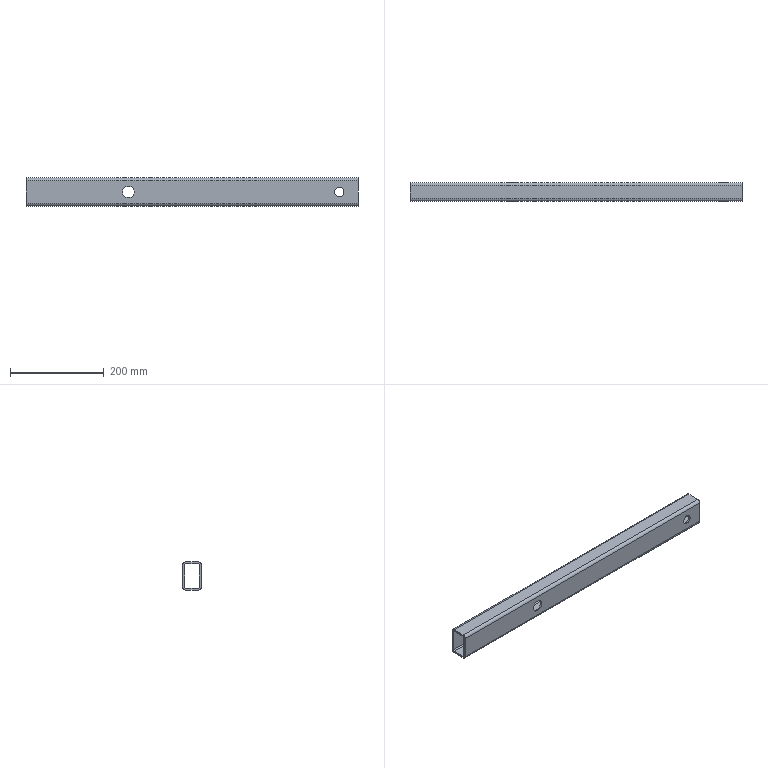Part | STEP file | 40 x 60 x 710 -2_Default<Machined> | 1 solid | 26 faces | box 710 x 40 x 60 mm | volume 494666 mm3 | cylinder 16 | plane 10 | commonest cylinder face diameters 4.8 x4 12.8 x4 20 x4 25 x4
STEP:
#1=CARTESIAN_POINT('',(82.078,-20.,-10.));
#2=VERTEX_POINT('',#1);
#3=CARTESIAN_POINT('',(82.078,-20.,10.));
#4=VERTEX_POINT('',#3);
#5=CARTESIAN_POINT('',(82.078,-20.,0.));
#6=DIRECTION('',(0.,1.,0.));
#7=DIRECTION('',(0.,0.,1.));
#8=AXIS2_PLACEMENT_3D('',#5,#6,#7);
#9=CIRCLE('',#8,10.);
#10=EDGE_CURVE('',#2,#4,#9,.T.);
#11=ORIENTED_EDGE('',*,*,#10,.F.);
#12=CARTESIAN_POINT('',(82.078,-16.,-10.));
#13=VERTEX_POINT('',#12);
#14=CARTESIAN_POINT('',(82.078,-20.,-10.));
#15=DIRECTION('',(0.,1.,0.));
#16=VECTOR('',#15,1000.);
#17=LINE('',#14,#16);
#18=EDGE_CURVE('',#2,#13,#17,.T.);
#19=ORIENTED_EDGE('',*,*,#18,.T.);
#20=CARTESIAN_POINT('',(82.078,-16.,10.));
#21=VERTEX_POINT('',#20);
#22=CARTESIAN_POINT('',(82.078,-16.,0.));
#23=DIRECTION('',(0.,1.,0.));
#24=DIRECTION('',(0.,0.,1.));
#25=AXIS2_PLACEMENT_3D('',#22,#23,#24);
#26=CIRCLE('',#25,10.);
#27=EDGE_CURVE('',#13,#21,#26,.T.);
#28=ORIENTED_EDGE('',*,*,#27,.T.);
#29=CARTESIAN_POINT('',(82.078,-20.,10.));
#30=DIRECTION('',(0.,1.,0.));
#31=VECTOR('',#30,1000.);
#32=LINE('',#29,#31);
#33=EDGE_CURVE('',#4,#21,#32,.T.);
#34=ORIENTED_EDGE('',*,*,#33,.F.);
#35=EDGE_LOOP('',(#11,#19,#28,#34));
#36=FACE_OUTER_BOUND('',#35,.T.);
#37=CARTESIAN_POINT('',(82.078,-20.,0.));
#38=DIRECTION('',(0.,1.,0.));
#39=DIRECTION('',(0.,0.,1.));
#40=AXIS2_PLACEMENT_3D('',#37,#38,#39);
#41=CYLINDRICAL_SURFACE('',#40,10.);
#42=ADVANCED_FACE('',(#36),#41,.F.);
#43=CARTESIAN_POINT('',(82.078,16.,10.));
#44=VERTEX_POINT('',#43);
#45=CARTESIAN_POINT('',(82.078,16.,-10.));
#46=VERTEX_POINT('',#45);
#47=CARTESIAN_POINT('',(82.078,16.,0.));
#48=DIRECTION('',(0.,-1.,0.));
#49=DIRECTION('',(0.,0.,-1.));
#50=AXIS2_PLACEMENT_3D('',#47,#48,#49);
#51=CIRCLE('',#50,10.);
#52=EDGE_CURVE('',#44,#46,#51,.T.);
#53=ORIENTED_EDGE('',*,*,#52,.T.);
#54=CARTESIAN_POINT('',(82.078,20.,-10.));
#55=VERTEX_POINT('',#54);
#56=CARTESIAN_POINT('',(82.078,-20.,-10.));
#57=DIRECTION('',(0.,1.,0.));
#58=VECTOR('',#57,1000.);
#59=LINE('',#56,#58);
#60=EDGE_CURVE('',#46,#55,#59,.T.);
#61=ORIENTED_EDGE('',*,*,#60,.T.);
#62=CARTESIAN_POINT('',(82.078,20.,10.));
#63=VERTEX_POINT('',#62);
#64=CARTESIAN_POINT('',(82.078,20.,0.));
#65=DIRECTION('',(0.,1.,0.));
#66=DIRECTION('',(0.,0.,1.));
#67=AXIS2_PLACEMENT_3D('',#64,#65,#66);
#68=CIRCLE('',#67,10.);
#69=EDGE_CURVE('',#55,#63,#68,.T.);
#70=ORIENTED_EDGE('',*,*,#69,.T.);
#71=CARTESIAN_POINT('',(82.078,-20.,10.));
#72=DIRECTION('',(0.,1.,0.));
#73=VECTOR('',#72,1000.);
#74=LINE('',#71,#73);
#75=EDGE_CURVE('',#44,#63,#74,.T.);
#76=ORIENTED_EDGE('',*,*,#75,.F.);
#77=EDGE_LOOP('',(#53,#61,#70,#76));
#78=FACE_OUTER_BOUND('',#77,.T.);
#79=CARTESIAN_POINT('',(82.078,-20.,0.));
#80=DIRECTION('',(0.,1.,0.));
#81=DIRECTION('',(0.,0.,1.));
#82=AXIS2_PLACEMENT_3D('',#79,#80,#81);
#83=CYLINDRICAL_SURFACE('',#82,10.);
#84=ADVANCED_FACE('',(#78),#83,.F.);
#85=CARTESIAN_POINT('',(-368.922,-20.,-12.5));
#86=VERTEX_POINT('',#85);
#87=CARTESIAN_POINT('',(-368.922,-20.,12.5));
#88=VERTEX_POINT('',#87);
#89=CARTESIAN_POINT('',(-368.922,-20.,0.));
#90=DIRECTION('',(0.,1.,0.));
#91=DIRECTION('',(0.,0.,1.));
#92=AXIS2_PLACEMENT_3D('',#89,#90,#91);
#93=CIRCLE('',#92,12.5);
#94=EDGE_CURVE('',#86,#88,#93,.T.);
#95=ORIENTED_EDGE('',*,*,#94,.F.);
#96=CARTESIAN_POINT('',(-368.922,-16.,-12.5));
#97=VERTEX_POINT('',#96);
#98=CARTESIAN_POINT('',(-368.922,-20.,-12.5));
#99=DIRECTION('',(0.,1.,0.));
#100=VECTOR('',#99,1000.);
#101=LINE('',#98,#100);
#102=EDGE_CURVE('',#86,#97,#101,.T.);
#103=ORIENTED_EDGE('',*,*,#102,.T.);
#104=CARTESIAN_POINT('',(-368.922,-16.,12.5));
#105=VERTEX_POINT('',#104);
#106=CARTESIAN_POINT('',(-368.922,-16.,0.));
#107=DIRECTION('',(0.,1.,0.));
#108=DIRECTION('',(0.,0.,1.));
#109=AXIS2_PLACEMENT_3D('',#106,#107,#108);
#110=CIRCLE('',#109,12.5);
#111=EDGE_CURVE('',#97,#105,#110,.T.);
#112=ORIENTED_EDGE('',*,*,#111,.T.);
#113=CARTESIAN_POINT('',(-368.922,-20.,12.5));
#114=DIRECTION('',(0.,1.,0.));
#115=VECTOR('',#114,1000.);
#116=LINE('',#113,#115);
#117=EDGE_CURVE('',#88,#105,#116,.T.);
#118=ORIENTED_EDGE('',*,*,#117,.F.);
#119=EDGE_LOOP('',(#95,#103,#112,#118));
#120=FACE_OUTER_BOUND('',#119,.T.);
#121=CARTESIAN_POINT('',(-368.922,-20.,0.));
#122=DIRECTION('',(0.,1.,0.));
#123=DIRECTION('',(0.,0.,1.));
#124=AXIS2_PLACEMENT_3D('',#121,#122,#123);
#125=CYLINDRICAL_SURFACE('',#124,12.5);
#126=ADVANCED_FACE('',(#120),#125,.F.);
#127=CARTESIAN_POINT('',(-368.922,16.,12.5));
#128=VERTEX_POINT('',#127);
#129=CARTESIAN_POINT('',(-368.922,16.,-12.5));
#130=VERTEX_POINT('',#129);
#131=CARTESIAN_POINT('',(-368.922,16.,0.));
#132=DIRECTION('',(0.,-1.,0.));
#133=DIRECTION('',(0.,0.,-1.));
#134=AXIS2_PLACEMENT_3D('',#131,#132,#133);
#135=CIRCLE('',#134,12.5);
#136=EDGE_CURVE('',#128,#130,#135,.T.);
#137=ORIENTED_EDGE('',*,*,#136,.T.);
#138=CARTESIAN_POINT('',(-368.922,20.,-12.5));
#139=VERTEX_POINT('',#138);
#140=CARTESIAN_POINT('',(-368.922,-20.,-12.5));
#141=DIRECTION('',(0.,1.,0.));
#142=VECTOR('',#141,1000.);
#143=LINE('',#140,#142);
#144=EDGE_CURVE('',#130,#139,#143,.T.);
#145=ORIENTED_EDGE('',*,*,#144,.T.);
#146=CARTESIAN_POINT('',(-368.922,20.,12.5));
#147=VERTEX_POINT('',#146);
#148=CARTESIAN_POINT('',(-368.922,20.,0.));
#149=DIRECTION('',(0.,1.,0.));
#150=DIRECTION('',(0.,0.,1.));
#151=AXIS2_PLACEMENT_3D('',#148,#149,#150);
#152=CIRCLE('',#151,12.5);
#153=EDGE_CURVE('',#139,#147,#152,.T.);
#154=ORIENTED_EDGE('',*,*,#153,.T.);
#155=CARTESIAN_POINT('',(-368.922,-20.,12.5));
#156=DIRECTION('',(0.,1.,0.));
#157=VECTOR('',#156,1000.);
#158=LINE('',#155,#157);
#159=EDGE_CURVE('',#128,#147,#158,.T.);
#160=ORIENTED_EDGE('',*,*,#159,.F.);
#161=EDGE_LOOP('',(#137,#145,#154,#160));
#162=FACE_OUTER_BOUND('',#161,.T.);
#163=CARTESIAN_POINT('',(-368.922,-20.,0.));
#164=DIRECTION('',(0.,1.,0.));
#165=DIRECTION('',(0.,0.,1.));
#166=AXIS2_PLACEMENT_3D('',#163,#164,#165);
#167=CYLINDRICAL_SURFACE('',#166,12.5);
#168=ADVANCED_FACE('',(#162),#167,.F.);
#169=CARTESIAN_POINT('',(-587.922,20.,23.6));
#170=VERTEX_POINT('',#169);
#171=CARTESIAN_POINT('',(-587.922,13.6,30.));
#172=VERTEX_POINT('',#171);
#173=CARTESIAN_POINT('',(-587.922,13.6,23.6));
#174=DIRECTION('',(1.,0.,0.));
#175=DIRECTION('',(0.,0.,-1.));
#176=AXIS2_PLACEMENT_3D('',#173,#174,#175);
#177=CIRCLE('',#176,6.4);
#178=EDGE_CURVE('',#170,#172,#177,.T.);
#179=ORIENTED_EDGE('',*,*,#178,.T.);
#180=CARTESIAN_POINT('',(122.078,13.6,30.));
#181=VERTEX_POINT('',#180);
#182=CARTESIAN_POINT('',(122.078,13.6,30.));
#183=DIRECTION('',(-1.,0.,0.));
#184=VECTOR('',#183,1000.);
#185=LINE('',#182,#184);
#186=EDGE_CURVE('',#181,#172,#185,.T.);
#187=ORIENTED_EDGE('',*,*,#186,.F.);
#188=CARTESIAN_POINT('',(122.078,20.,23.6));
#189=VERTEX_POINT('',#188);
#190=CARTESIAN_POINT('',(122.078,13.6,23.6));
#191=DIRECTION('',(1.,0.,0.));
#192=DIRECTION('',(0.,0.,-1.));
#193=AXIS2_PLACEMENT_3D('',#190,#191,#192);
#194=CIRCLE('',#193,6.4);
#195=EDGE_CURVE('',#189,#181,#194,.T.);
#196=ORIENTED_EDGE('',*,*,#195,.F.);
#197=CARTESIAN_POINT('',(122.078,20.,23.6));
#198=DIRECTION('',(-1.,0.,0.));
#199=VECTOR('',#198,1000.);
#200=LINE('',#197,#199);
#201=EDGE_CURVE('',#189,#170,#200,.T.);
#202=ORIENTED_EDGE('',*,*,#201,.T.);
#203=EDGE_LOOP('',(#179,#187,#196,#202));
#204=FACE_OUTER_BOUND('',#203,.T.);
#205=CARTESIAN_POINT('',(122.078,13.6,23.6));
#206=DIRECTION('',(-1.,0.,0.));
#207=DIRECTION('',(0.,0.,1.));
#208=AXIS2_PLACEMENT_3D('',#205,#206,#207);
#209=CYLINDRICAL_SURFACE('',#208,6.4);
#210=ADVANCED_FACE('',(#204),#209,.T.);
#211=CARTESIAN_POINT('',(-587.922,-13.6,30.));
#212=VERTEX_POINT('',#211);
#213=CARTESIAN_POINT('',(-587.922,13.6,30.));
#214=DIRECTION('',(0.,-1.,0.));
#215=VECTOR('',#214,1000.);
#216=LINE('',#213,#215);
#217=EDGE_CURVE('',#172,#212,#216,.T.);
#218=ORIENTED_EDGE('',*,*,#217,.T.);
#219=CARTESIAN_POINT('',(122.078,-13.6,30.));
#220=VERTEX_POINT('',#219);
#221=CARTESIAN_POINT('',(122.078,-13.6,30.));
#222=DIRECTION('',(-1.,0.,0.));
#223=VECTOR('',#222,1000.);
#224=LINE('',#221,#223);
#225=EDGE_CURVE('',#220,#212,#224,.T.);
#226=ORIENTED_EDGE('',*,*,#225,.F.);
#227=CARTESIAN_POINT('',(122.078,13.6,30.));
#228=DIRECTION('',(0.,-1.,0.));
#229=VECTOR('',#228,1000.);
#230=LINE('',#227,#229);
#231=EDGE_CURVE('',#181,#220,#230,.T.);
#232=ORIENTED_EDGE('',*,*,#231,.F.);
#233=ORIENTED_EDGE('',*,*,#186,.T.);
#234=EDGE_LOOP('',(#218,#226,#232,#233));
#235=FACE_OUTER_BOUND('',#234,.T.);
#236=CARTESIAN_POINT('',(122.078,13.6,30.));
#237=DIRECTION('',(0.,0.,-1.));
#238=DIRECTION('',(-1.,0.,0.));
#239=AXIS2_PLACEMENT_3D('',#236,#237,#238);
#240=PLANE('',#239);
#241=ADVANCED_FACE('',(#235),#240,.F.);
#242=CARTESIAN_POINT('',(-587.922,-20.,23.6));
#243=VERTEX_POINT('',#242);
#244=CARTESIAN_POINT('',(-587.922,-13.6,23.6));
#245=DIRECTION('',(1.,0.,0.));
#246=DIRECTION('',(0.,0.,-1.));
#247=AXIS2_PLACEMENT_3D('',#244,#245,#246);
#248=CIRCLE('',#247,6.4);
#249=EDGE_CURVE('',#212,#243,#248,.T.);
#250=ORIENTED_EDGE('',*,*,#249,.T.);
#251=CARTESIAN_POINT('',(122.078,-20.,23.6));
#252=VERTEX_POINT('',#251);
#253=CARTESIAN_POINT('',(122.078,-20.,23.6));
#254=DIRECTION('',(-1.,0.,0.));
#255=VECTOR('',#254,1000.);
#256=LINE('',#253,#255);
#257=EDGE_CURVE('',#252,#243,#256,.T.);
#258=ORIENTED_EDGE('',*,*,#257,.F.);
#259=CARTESIAN_POINT('',(122.078,-13.6,23.6));
#260=DIRECTION('',(1.,0.,0.));
#261=DIRECTION('',(0.,0.,-1.));
#262=AXIS2_PLACEMENT_3D('',#259,#260,#261);
#263=CIRCLE('',#262,6.4);
#264=EDGE_CURVE('',#220,#252,#263,.T.);
#265=ORIENTED_EDGE('',*,*,#264,.F.);
#266=ORIENTED_EDGE('',*,*,#225,.T.);
#267=EDGE_LOOP('',(#250,#258,#265,#266));
#268=FACE_OUTER_BOUND('',#267,.T.);
#269=CARTESIAN_POINT('',(122.078,-13.6,23.6));
#270=DIRECTION('',(-1.,0.,0.));
#271=DIRECTION('',(0.,0.,1.));
#272=AXIS2_PLACEMENT_3D('',#269,#270,#271);
#273=CYLINDRICAL_SURFACE('',#272,6.4);
#274=ADVANCED_FACE('',(#268),#273,.T.);
#275=CARTESIAN_POINT('',(82.078,-20.,0.));
#276=DIRECTION('',(0.,1.,0.));
#277=DIRECTION('',(0.,0.,1.));
#278=AXIS2_PLACEMENT_3D('',#275,#276,#277);
#279=CIRCLE('',#278,10.);
#280=EDGE_CURVE('',#4,#2,#279,.T.);
#281=ORIENTED_EDGE('',*,*,#280,.T.);
#282=ORIENTED_EDGE('',*,*,#10,.T.);
#283=EDGE_LOOP('',(#281,#282));
#284=FACE_BOUND('',#283,.T.);
#285=CARTESIAN_POINT('',(-368.922,-20.,0.));
#286=DIRECTION('',(0.,1.,0.));
#287=DIRECTION('',(0.,0.,1.));
#288=AXIS2_PLACEMENT_3D('',#285,#286,#287);
#289=CIRCLE('',#288,12.5);
#290=EDGE_CURVE('',#88,#86,#289,.T.);
#291=ORIENTED_EDGE('',*,*,#290,.T.);
#292=ORIENTED_EDGE('',*,*,#94,.T.);
#293=EDGE_LOOP('',(#291,#292));
#294=FACE_BOUND('',#293,.T.);
#295=CARTESIAN_POINT('',(-587.922,-20.,-23.6));
#296=VERTEX_POINT('',#295);
#297=CARTESIAN_POINT('',(-587.922,-20.,-23.6));
#298=DIRECTION('',(0.,0.,-1.));
#299=VECTOR('',#298,1000.);
#300=LINE('',#297,#299);
#301=EDGE_CURVE('',#243,#296,#300,.T.);
#302=ORIENTED_EDGE('',*,*,#301,.T.);
#303=CARTESIAN_POINT('',(122.078,-20.,-23.6));
#304=VERTEX_POINT('',#303);
#305=CARTESIAN_POINT('',(122.078,-20.,-23.6));
#306=DIRECTION('',(-1.,0.,0.));
#307=VECTOR('',#306,1000.);
#308=LINE('',#305,#307);
#309=EDGE_CURVE('',#304,#296,#308,.T.);
#310=ORIENTED_EDGE('',*,*,#309,.F.);
#311=CARTESIAN_POINT('',(122.078,-20.,-23.6));
#312=DIRECTION('',(0.,0.,-1.));
#313=VECTOR('',#312,1000.);
#314=LINE('',#311,#313);
#315=EDGE_CURVE('',#252,#304,#314,.T.);
#316=ORIENTED_EDGE('',*,*,#315,.F.);
#317=ORIENTED_EDGE('',*,*,#257,.T.);
#318=EDGE_LOOP('',(#302,#310,#316,#317));
#319=FACE_OUTER_BOUND('',#318,.T.);
#320=CARTESIAN_POINT('',(122.078,-20.,-23.6));
#321=DIRECTION('',(0.,1.,0.));
#322=DIRECTION('',(0.,0.,1.));
#323=AXIS2_PLACEMENT_3D('',#320,#321,#322);
#324=PLANE('',#323);
#325=ADVANCED_FACE('',(#284,#294,#319),#324,.F.);
#326=CARTESIAN_POINT('',(-587.922,-13.6,-30.));
#327=VERTEX_POINT('',#326);
#328=CARTESIAN_POINT('',(-587.922,-13.6,-23.6));
#329=DIRECTION('',(1.,0.,0.));
#330=DIRECTION('',(0.,0.,-1.));
#331=AXIS2_PLACEMENT_3D('',#328,#329,#330);
#332=CIRCLE('',#331,6.4);
#333=EDGE_CURVE('',#296,#327,#332,.T.);
#334=ORIENTED_EDGE('',*,*,#333,.T.);
#335=CARTESIAN_POINT('',(122.078,-13.6,-30.));
#336=VERTEX_POINT('',#335);
#337=CARTESIAN_POINT('',(122.078,-13.6,-30.));
#338=DIRECTION('',(-1.,0.,0.));
#339=VECTOR('',#338,1000.);
#340=LINE('',#337,#339);
#341=EDGE_CURVE('',#336,#327,#340,.T.);
#342=ORIENTED_EDGE('',*,*,#341,.F.);
#343=CARTESIAN_POINT('',(122.078,-13.6,-23.6));
#344=DIRECTION('',(1.,0.,0.));
#345=DIRECTION('',(0.,0.,-1.));
#346=AXIS2_PLACEMENT_3D('',#343,#344,#345);
#347=CIRCLE('',#346,6.4);
#348=EDGE_CURVE('',#304,#336,#347,.T.);
#349=ORIENTED_EDGE('',*,*,#348,.F.);
#350=ORIENTED_EDGE('',*,*,#309,.T.);
#351=EDGE_LOOP('',(#334,#342,#349,#350));
#352=FACE_OUTER_BOUND('',#351,.T.);
#353=CARTESIAN_POINT('',(122.078,-13.6,-23.6));
#354=DIRECTION('',(-1.,0.,0.));
#355=DIRECTION('',(0.,0.,1.));
#356=AXIS2_PLACEMENT_3D('',#353,#354,#355);
#357=CYLINDRICAL_SURFACE('',#356,6.4);
#358=ADVANCED_FACE('',(#352),#357,.T.);
#359=CARTESIAN_POINT('',(-587.922,13.6,-30.));
#360=VERTEX_POINT('',#359);
#361=CARTESIAN_POINT('',(-587.922,-13.6,-30.));
#362=DIRECTION('',(0.,1.,0.));
#363=VECTOR('',#362,1000.);
#364=LINE('',#361,#363);
#365=EDGE_CURVE('',#327,#360,#364,.T.);
#366=ORIENTED_EDGE('',*,*,#365,.T.);
#367=CARTESIAN_POINT('',(122.078,13.6,-30.));
#368=VERTEX_POINT('',#367);
#369=CARTESIAN_POINT('',(122.078,13.6,-30.));
#370=DIRECTION('',(-1.,0.,0.));
#371=VECTOR('',#370,1000.);
#372=LINE('',#369,#371);
#373=EDGE_CURVE('',#368,#360,#372,.T.);
#374=ORIENTED_EDGE('',*,*,#373,.F.);
#375=CARTESIAN_POINT('',(122.078,-13.6,-30.));
#376=DIRECTION('',(0.,1.,0.));
#377=VECTOR('',#376,1000.);
#378=LINE('',#375,#377);
#379=EDGE_CURVE('',#336,#368,#378,.T.);
#380=ORIENTED_EDGE('',*,*,#379,.F.);
#381=ORIENTED_EDGE('',*,*,#341,.T.);
#382=EDGE_LOOP('',(#366,#374,#380,#381));
#383=FACE_OUTER_BOUND('',#382,.T.);
#384=CARTESIAN_POINT('',(122.078,-13.6,-30.));
#385=DIRECTION('',(0.,0.,1.));
#386=DIRECTION('',(1.,0.,0.));
#387=AXIS2_PLACEMENT_3D('',#384,#385,#386);
#388=PLANE('',#387);
#389=ADVANCED_FACE('',(#383),#388,.F.);
#390=CARTESIAN_POINT('',(-587.922,20.,-23.6));
#391=VERTEX_POINT('',#390);
#392=CARTESIAN_POINT('',(-587.922,13.6,-23.6));
#393=DIRECTION('',(1.,0.,0.));
#394=DIRECTION('',(0.,0.,-1.));
#395=AXIS2_PLACEMENT_3D('',#392,#393,#394);
#396=CIRCLE('',#395,6.4);
#397=EDGE_CURVE('',#360,#391,#396,.T.);
#398=ORIENTED_EDGE('',*,*,#397,.T.);
#399=CARTESIAN_POINT('',(122.078,20.,-23.6));
#400=VERTEX_POINT('',#399);
#401=CARTESIAN_POINT('',(122.078,20.,-23.6));
#402=DIRECTION('',(-1.,0.,0.));
#403=VECTOR('',#402,1000.);
#404=LINE('',#401,#403);
#405=EDGE_CURVE('',#400,#391,#404,.T.);
#406=ORIENTED_EDGE('',*,*,#405,.F.);
#407=CARTESIAN_POINT('',(122.078,13.6,-23.6));
#408=DIRECTION('',(1.,0.,0.));
#409=DIRECTION('',(0.,0.,-1.));
#410=AXIS2_PLACEMENT_3D('',#407,#408,#409);
#411=CIRCLE('',#410,6.4);
#412=EDGE_CURVE('',#368,#400,#411,.T.);
#413=ORIENTED_EDGE('',*,*,#412,.F.);
#414=ORIENTED_EDGE('',*,*,#373,.T.);
#415=EDGE_LOOP('',(#398,#406,#413,#414));
#416=FACE_OUTER_BOUND('',#415,.T.);
#417=CARTESIAN_POINT('',(122.078,13.6,-23.6));
#418=DIRECTION('',(-1.,0.,0.));
#419=DIRECTION('',(0.,0.,1.));
#420=AXIS2_PLACEMENT_3D('',#417,#418,#419);
#421=CYLINDRICAL_SURFACE('',#420,6.4);
#422=ADVANCED_FACE('',(#416),#421,.T.);
#423=CARTESIAN_POINT('',(-587.922,-13.6,26.));
#424=VERTEX_POINT('',#423);
#425=CARTESIAN_POINT('',(-587.922,-16.,23.6));
#426=VERTEX_POINT('',#425);
#427=CARTESIAN_POINT('',(-587.922,-13.6,23.6));
#428=DIRECTION('',(1.,0.,0.));
#429=DIRECTION('',(0.,0.,-1.));
#430=AXIS2_PLACEMENT_3D('',#427,#428,#429);
#431=CIRCLE('',#430,2.4);
#432=EDGE_CURVE('',#424,#426,#431,.T.);
#433=ORIENTED_EDGE('',*,*,#432,.F.);
#434=CARTESIAN_POINT('',(122.078,-13.6,26.));
#435=VERTEX_POINT('',#434);
#436=CARTESIAN_POINT('',(122.078,-13.6,26.));
#437=DIRECTION('',(-1.,0.,0.));
#438=VECTOR('',#437,1000.);
#439=LINE('',#436,#438);
#440=EDGE_CURVE('',#435,#424,#439,.T.);
#441=ORIENTED_EDGE('',*,*,#440,.F.);
#442=CARTESIAN_POINT('',(122.078,-16.,23.6));
#443=VERTEX_POINT('',#442);
#444=CARTESIAN_POINT('',(122.078,-13.6,23.6));
#445=DIRECTION('',(1.,0.,0.));
#446=DIRECTION('',(0.,0.,-1.));
#447=AXIS2_PLACEMENT_3D('',#444,#445,#446);
#448=CIRCLE('',#447,2.4);
#449=EDGE_CURVE('',#435,#443,#448,.T.);
#450=ORIENTED_EDGE('',*,*,#449,.T.);
#451=CARTESIAN_POINT('',(122.078,-16.,23.6));
#452=DIRECTION('',(-1.,0.,0.));
#453=VECTOR('',#452,1000.);
#454=LINE('',#451,#453);
#455=EDGE_CURVE('',#443,#426,#454,.T.);
#456=ORIENTED_EDGE('',*,*,#455,.T.);
#457=EDGE_LOOP('',(#433,#441,#450,#456));
#458=FACE_OUTER_BOUND('',#457,.T.);
#459=CARTESIAN_POINT('',(122.078,-13.6,23.6));
#460=DIRECTION('',(-1.,0.,0.));
#461=DIRECTION('',(0.,0.,1.));
#462=AXIS2_PLACEMENT_3D('',#459,#460,#461);
#463=CYLINDRICAL_SURFACE('',#462,2.4);
#464=ADVANCED_FACE('',(#458),#463,.F.);
#465=CARTESIAN_POINT('',(-587.922,13.6,26.));
#466=VERTEX_POINT('',#465);
#467=CARTESIAN_POINT('',(-587.922,13.6,26.));
#468=DIRECTION('',(0.,-1.,0.));
#469=VECTOR('',#468,1000.);
#470=LINE('',#467,#469);
#471=EDGE_CURVE('',#466,#424,#470,.T.);
#472=ORIENTED_EDGE('',*,*,#471,.F.);
#473=CARTESIAN_POINT('',(122.078,13.6,26.));
#474=VERTEX_POINT('',#473);
#475=CARTESIAN_POINT('',(122.078,13.6,26.));
#476=DIRECTION('',(-1.,0.,0.));
#477=VECTOR('',#476,1000.);
#478=LINE('',#475,#477);
#479=EDGE_CURVE('',#474,#466,#478,.T.);
#480=ORIENTED_EDGE('',*,*,#479,.F.);
#481=CARTESIAN_POINT('',(122.078,13.6,26.));
#482=DIRECTION('',(0.,-1.,0.));
#483=VECTOR('',#482,1000.);
#484=LINE('',#481,#483);
#485=EDGE_CURVE('',#474,#435,#484,.T.);
#486=ORIENTED_EDGE('',*,*,#485,.T.);
#487=ORIENTED_EDGE('',*,*,#440,.T.);
#488=EDGE_LOOP('',(#472,#480,#486,#487));
#489=FACE_OUTER_BOUND('',#488,.T.);
#490=CARTESIAN_POINT('',(122.078,13.6,26.));
#491=DIRECTION('',(0.,0.,-1.));
#492=DIRECTION('',(-1.,0.,0.));
#493=AXIS2_PLACEMENT_3D('',#490,#491,#492);
#494=PLANE('',#493);
#495=ADVANCED_FACE('',(#489),#494,.T.);
#496=CARTESIAN_POINT('',(-587.922,16.,23.6));
#497=VERTEX_POINT('',#496);
#498=CARTESIAN_POINT('',(-587.922,13.6,23.6));
#499=DIRECTION('',(1.,0.,0.));
#500=DIRECTION('',(0.,0.,-1.));
#501=AXIS2_PLACEMENT_3D('',#498,#499,#500);
#502=CIRCLE('',#501,2.4);
#503=EDGE_CURVE('',#497,#466,#502,.T.);
#504=ORIENTED_EDGE('',*,*,#503,.F.);
#505=CARTESIAN_POINT('',(122.078,16.,23.6));
#506=VERTEX_POINT('',#505);
#507=CARTESIAN_POINT('',(122.078,16.,23.6));
#508=DIRECTION('',(-1.,0.,0.));
#509=VECTOR('',#508,1000.);
#510=LINE('',#507,#509);
#511=EDGE_CURVE('',#506,#497,#510,.T.);
#512=ORIENTED_EDGE('',*,*,#511,.F.);
#513=CARTESIAN_POINT('',(122.078,13.6,23.6));
#514=DIRECTION('',(1.,0.,0.));
#515=DIRECTION('',(0.,0.,-1.));
#516=AXIS2_PLACEMENT_3D('',#513,#514,#515);
#517=CIRCLE('',#516,2.4);
#518=EDGE_CURVE('',#506,#474,#517,.T.);
#519=ORIENTED_EDGE('',*,*,#518,.T.);
#520=ORIENTED_EDGE('',*,*,#479,.T.);
#521=EDGE_LOOP('',(#504,#512,#519,#520));
#522=FACE_OUTER_BOUND('',#521,.T.);
#523=CARTESIAN_POINT('',(122.078,13.6,23.6));
#524=DIRECTION('',(-1.,0.,0.));
#525=DIRECTION('',(0.,0.,1.));
#526=AXIS2_PLACEMENT_3D('',#523,#524,#525);
#527=CYLINDRICAL_SURFACE('',#526,2.4);
#528=ADVANCED_FACE('',(#522),#527,.F.);
#529=ORIENTED_EDGE('',*,*,#52,.F.);
#530=CARTESIAN_POINT('',(82.078,16.,0.));
#531=DIRECTION('',(0.,-1.,0.));
#532=DIRECTION('',(0.,0.,-1.));
#533=AXIS2_PLACEMENT_3D('',#530,#531,#532);
#534=CIRCLE('',#533,10.);
#535=EDGE_CURVE('',#46,#44,#534,.T.);
#536=ORIENTED_EDGE('',*,*,#535,.F.);
#537=EDGE_LOOP('',(#529,#536));
#538=FACE_BOUND('',#537,.T.);
#539=ORIENTED_EDGE('',*,*,#136,.F.);
#540=CARTESIAN_POINT('',(-368.922,16.,0.));
#541=DIRECTION('',(0.,-1.,0.));
#542=DIRECTION('',(0.,0.,-1.));
#543=AXIS2_PLACEMENT_3D('',#540,#541,#542);
#544=CIRCLE('',#543,12.5);
#545=EDGE_CURVE('',#130,#128,#544,.T.);
#546=ORIENTED_EDGE('',*,*,#545,.F.);
#547=EDGE_LOOP('',(#539,#546));
#548=FACE_BOUND('',#547,.T.);
#549=CARTESIAN_POINT('',(-587.922,16.,-23.6));
#550=VERTEX_POINT('',#549);
#551=CARTESIAN_POINT('',(-587.922,16.,23.6));
#552=DIRECTION('',(0.,0.,1.));
#553=VECTOR('',#552,1000.);
#554=LINE('',#551,#553);
#555=EDGE_CURVE('',#550,#497,#554,.T.);
#556=ORIENTED_EDGE('',*,*,#555,.F.);
#557=CARTESIAN_POINT('',(122.078,16.,-23.6));
#558=VERTEX_POINT('',#557);
#559=CARTESIAN_POINT('',(122.078,16.,-23.6));
#560=DIRECTION('',(-1.,0.,0.));
#561=VECTOR('',#560,1000.);
#562=LINE('',#559,#561);
#563=EDGE_CURVE('',#558,#550,#562,.T.);
#564=ORIENTED_EDGE('',*,*,#563,.F.);
#565=CARTESIAN_POINT('',(122.078,16.,23.6));
#566=DIRECTION('',(0.,0.,1.));
#567=VECTOR('',#566,1000.);
#568=LINE('',#565,#567);
#569=EDGE_CURVE('',#558,#506,#568,.T.);
#570=ORIENTED_EDGE('',*,*,#569,.T.);
#571=ORIENTED_EDGE('',*,*,#511,.T.);
#572=EDGE_LOOP('',(#556,#564,#570,#571));
#573=FACE_OUTER_BOUND('',#572,.T.);
#574=CARTESIAN_POINT('',(122.078,16.,23.6));
#575=DIRECTION('',(0.,-1.,0.));
#576=DIRECTION('',(0.,0.,-1.));
#577=AXIS2_PLACEMENT_3D('',#574,#575,#576);
#578=PLANE('',#577);
#579=ADVANCED_FACE('',(#538,#548,#573),#578,.T.);
#580=CARTESIAN_POINT('',(-587.922,13.6,-26.));
#581=VERTEX_POINT('',#580);
#582=CARTESIAN_POINT('',(-587.922,13.6,-23.6));
#583=DIRECTION('',(1.,0.,0.));
#584=DIRECTION('',(0.,0.,-1.));
#585=AXIS2_PLACEMENT_3D('',#582,#583,#584);
#586=CIRCLE('',#585,2.4);
#587=EDGE_CURVE('',#581,#550,#586,.T.);
#588=ORIENTED_EDGE('',*,*,#587,.F.);
#589=CARTESIAN_POINT('',(122.078,13.6,-26.));
#590=VERTEX_POINT('',#589);
#591=CARTESIAN_POINT('',(122.078,13.6,-26.));
#592=DIRECTION('',(-1.,0.,0.));
#593=VECTOR('',#592,1000.);
#594=LINE('',#591,#593);
#595=EDGE_CURVE('',#590,#581,#594,.T.);
#596=ORIENTED_EDGE('',*,*,#595,.F.);
#597=CARTESIAN_POINT('',(122.078,13.6,-23.6));
#598=DIRECTION('',(1.,0.,0.));
#599=DIRECTION('',(0.,0.,-1.));
#600=AXIS2_PLACEMENT_3D('',#597,#598,#599);
#601=CIRCLE('',#600,2.4);
#602=EDGE_CURVE('',#590,#558,#601,.T.);
#603=ORIENTED_EDGE('',*,*,#602,.T.);
#604=ORIENTED_EDGE('',*,*,#563,.T.);
#605=EDGE_LOOP('',(#588,#596,#603,#604));
#606=FACE_OUTER_BOUND('',#605,.T.);
#607=CARTESIAN_POINT('',(122.078,13.6,-23.6));
#608=DIRECTION('',(-1.,0.,0.));
#609=DIRECTION('',(0.,0.,1.));
#610=AXIS2_PLACEMENT_3D('',#607,#608,#609);
#611=CYLINDRICAL_SURFACE('',#610,2.4);
#612=ADVANCED_FACE('',(#606),#611,.F.);
#613=CARTESIAN_POINT('',(-587.922,-13.6,-26.));
#614=VERTEX_POINT('',#613);
#615=CARTESIAN_POINT('',(-587.922,-13.6,-26.));
#616=DIRECTION('',(0.,1.,0.));
#617=VECTOR('',#616,1000.);
#618=LINE('',#615,#617);
#619=EDGE_CURVE('',#614,#581,#618,.T.);
#620=ORIENTED_EDGE('',*,*,#619,.F.);
#621=CARTESIAN_POINT('',(122.078,-13.6,-26.));
#622=VERTEX_POINT('',#621);
#623=CARTESIAN_POINT('',(122.078,-13.6,-26.));
#624=DIRECTION('',(-1.,0.,0.));
#625=VECTOR('',#624,1000.);
#626=LINE('',#623,#625);
#627=EDGE_CURVE('',#622,#614,#626,.T.);
#628=ORIENTED_EDGE('',*,*,#627,.F.);
#629=CARTESIAN_POINT('',(122.078,-13.6,-26.));
#630=DIRECTION('',(0.,1.,0.));
#631=VECTOR('',#630,1000.);
#632=LINE('',#629,#631);
#633=EDGE_CURVE('',#622,#590,#632,.T.);
#634=ORIENTED_EDGE('',*,*,#633,.T.);
#635=ORIENTED_EDGE('',*,*,#595,.T.);
#636=EDGE_LOOP('',(#620,#628,#634,#635));
#637=FACE_OUTER_BOUND('',#636,.T.);
#638=CARTESIAN_POINT('',(122.078,-13.6,-26.));
#639=DIRECTION('',(0.,0.,1.));
#640=DIRECTION('',(1.,0.,0.));
#641=AXIS2_PLACEMENT_3D('',#638,#639,#640);
#642=PLANE('',#641);
#643=ADVANCED_FACE('',(#637),#642,.T.);
#644=CARTESIAN_POINT('',(-587.922,-16.,-23.6));
#645=VERTEX_POINT('',#644);
#646=CARTESIAN_POINT('',(-587.922,-13.6,-23.6));
#647=DIRECTION('',(1.,0.,0.));
#648=DIRECTION('',(0.,0.,-1.));
#649=AXIS2_PLACEMENT_3D('',#646,#647,#648);
#650=CIRCLE('',#649,2.4);
#651=EDGE_CURVE('',#645,#614,#650,.T.);
#652=ORIENTED_EDGE('',*,*,#651,.F.);
#653=CARTESIAN_POINT('',(122.078,-16.,-23.6));
#654=VERTEX_POINT('',#653);
#655=CARTESIAN_POINT('',(122.078,-16.,-23.6));
#656=DIRECTION('',(-1.,0.,0.));
#657=VECTOR('',#656,1000.);
#658=LINE('',#655,#657);
#659=EDGE_CURVE('',#654,#645,#658,.T.);
#660=ORIENTED_EDGE('',*,*,#659,.F.);
#661=CARTESIAN_POINT('',(122.078,-13.6,-23.6));
#662=DIRECTION('',(1.,0.,0.));
#663=DIRECTION('',(0.,0.,-1.));
#664=AXIS2_PLACEMENT_3D('',#661,#662,#663);
#665=CIRCLE('',#664,2.4);
#666=EDGE_CURVE('',#654,#622,#665,.T.);
#667=ORIENTED_EDGE('',*,*,#666,.T.);
#668=ORIENTED_EDGE('',*,*,#627,.T.);
#669=EDGE_LOOP('',(#652,#660,#667,#668));
#670=FACE_OUTER_BOUND('',#669,.T.);
#671=CARTESIAN_POINT('',(122.078,-13.6,-23.6));
#672=DIRECTION('',(-1.,0.,0.));
#673=DIRECTION('',(0.,0.,1.));
#674=AXIS2_PLACEMENT_3D('',#671,#672,#673);
#675=CYLINDRICAL_SURFACE('',#674,2.4);
#676=ADVANCED_FACE('',(#670),#675,.F.);
#677=CARTESIAN_POINT('',(82.078,-16.,0.));
#678=DIRECTION('',(0.,1.,0.));
#679=DIRECTION('',(0.,0.,1.));
#680=AXIS2_PLACEMENT_3D('',#677,#678,#679);
#681=CIRCLE('',#680,10.);
#682=EDGE_CURVE('',#21,#13,#681,.T.);
#683=ORIENTED_EDGE('',*,*,#682,.F.);
#684=ORIENTED_EDGE('',*,*,#27,.F.);
#685=EDGE_LOOP('',(#683,#684));
#686=FACE_BOUND('',#685,.T.);
#687=CARTESIAN_POINT('',(-368.922,-16.,0.));
#688=DIRECTION('',(0.,1.,0.));
#689=DIRECTION('',(0.,0.,1.));
#690=AXIS2_PLACEMENT_3D('',#687,#688,#689);
#691=CIRCLE('',#690,12.5);
#692=EDGE_CURVE('',#105,#97,#691,.T.);
#693=ORIENTED_EDGE('',*,*,#692,.F.);
#694=ORIENTED_EDGE('',*,*,#111,.F.);
#695=EDGE_LOOP('',(#693,#694));
#696=FACE_BOUND('',#695,.T.);
#697=CARTESIAN_POINT('',(-587.922,-16.,-23.6));
#698=DIRECTION('',(0.,0.,-1.));
#699=VECTOR('',#698,1000.);
#700=LINE('',#697,#699);
#701=EDGE_CURVE('',#426,#645,#700,.T.);
#702=ORIENTED_EDGE('',*,*,#701,.F.);
#703=ORIENTED_EDGE('',*,*,#455,.F.);
#704=CARTESIAN_POINT('',(122.078,-16.,-23.6));
#705=DIRECTION('',(0.,0.,-1.));
#706=VECTOR('',#705,1000.);
#707=LINE('',#704,#706);
#708=EDGE_CURVE('',#443,#654,#707,.T.);
#709=ORIENTED_EDGE('',*,*,#708,.T.);
#710=ORIENTED_EDGE('',*,*,#659,.T.);
#711=EDGE_LOOP('',(#702,#703,#709,#710));
#712=FACE_OUTER_BOUND('',#711,.T.);
#713=CARTESIAN_POINT('',(122.078,-16.,-23.6));
#714=DIRECTION('',(0.,1.,0.));
#715=DIRECTION('',(0.,0.,1.));
#716=AXIS2_PLACEMENT_3D('',#713,#714,#715);
#717=PLANE('',#716);
#718=ADVANCED_FACE('',(#686,#696,#712),#717,.T.);
#719=CARTESIAN_POINT('',(82.078,20.,0.));
#720=DIRECTION('',(0.,1.,0.));
#721=DIRECTION('',(0.,0.,1.));
#722=AXIS2_PLACEMENT_3D('',#719,#720,#721);
#723=CIRCLE('',#722,10.);
#724=EDGE_CURVE('',#63,#55,#723,.T.);
#725=ORIENTED_EDGE('',*,*,#724,.F.);
#726=ORIENTED_EDGE('',*,*,#69,.F.);
#727=EDGE_LOOP('',(#725,#726));
#728=FACE_BOUND('',#727,.T.);
#729=CARTESIAN_POINT('',(-368.922,20.,0.));
#730=DIRECTION('',(0.,1.,0.));
#731=DIRECTION('',(0.,0.,1.));
#732=AXIS2_PLACEMENT_3D('',#729,#730,#731);
#733=CIRCLE('',#732,12.5);
#734=EDGE_CURVE('',#147,#139,#733,.T.);
#735=ORIENTED_EDGE('',*,*,#734,.F.);
#736=ORIENTED_EDGE('',*,*,#153,.F.);
#737=EDGE_LOOP('',(#735,#736));
#738=FACE_BOUND('',#737,.T.);
#739=CARTESIAN_POINT('',(-587.922,20.,23.6));
#740=DIRECTION('',(0.,0.,1.));
#741=VECTOR('',#740,1000.);
#742=LINE('',#739,#741);
#743=EDGE_CURVE('',#391,#170,#742,.T.);
#744=ORIENTED_EDGE('',*,*,#743,.T.);
#745=ORIENTED_EDGE('',*,*,#201,.F.);
#746=CARTESIAN_POINT('',(122.078,20.,23.6));
#747=DIRECTION('',(0.,0.,1.));
#748=VECTOR('',#747,1000.);
#749=LINE('',#746,#748);
#750=EDGE_CURVE('',#400,#189,#749,.T.);
#751=ORIENTED_EDGE('',*,*,#750,.F.);
#752=ORIENTED_EDGE('',*,*,#405,.T.);
#753=EDGE_LOOP('',(#744,#745,#751,#752));
#754=FACE_OUTER_BOUND('',#753,.T.);
#755=CARTESIAN_POINT('',(122.078,20.,23.6));
#756=DIRECTION('',(0.,-1.,0.));
#757=DIRECTION('',(0.,0.,-1.));
#758=AXIS2_PLACEMENT_3D('',#755,#756,#757);
#759=PLANE('',#758);
#760=ADVANCED_FACE('',(#728,#738,#754),#759,.F.);
#761=ORIENTED_EDGE('',*,*,#449,.F.);
#762=ORIENTED_EDGE('',*,*,#485,.F.);
#763=ORIENTED_EDGE('',*,*,#518,.F.);
#764=ORIENTED_EDGE('',*,*,#569,.F.);
#765=ORIENTED_EDGE('',*,*,#602,.F.);
#766=ORIENTED_EDGE('',*,*,#633,.F.);
#767=ORIENTED_EDGE('',*,*,#666,.F.);
#768=ORIENTED_EDGE('',*,*,#708,.F.);
#769=EDGE_LOOP('',(#761,#762,#763,#764,#765,#766,#767,#768));
#770=FACE_BOUND('',#769,.T.);
#771=ORIENTED_EDGE('',*,*,#195,.T.);
#772=ORIENTED_EDGE('',*,*,#231,.T.);
#773=ORIENTED_EDGE('',*,*,#264,.T.);
#774=ORIENTED_EDGE('',*,*,#315,.T.);
#775=ORIENTED_EDGE('',*,*,#348,.T.);
#776=ORIENTED_EDGE('',*,*,#379,.T.);
#777=ORIENTED_EDGE('',*,*,#412,.T.);
#778=ORIENTED_EDGE('',*,*,#750,.T.);
#779=EDGE_LOOP('',(#771,#772,#773,#774,#775,#776,#777,#778));
#780=FACE_OUTER_BOUND('',#779,.T.);
#781=CARTESIAN_POINT('',(122.078,13.6,23.6));
#782=DIRECTION('',(1.,0.,0.));
#783=DIRECTION('',(0.,0.,-1.));
#784=AXIS2_PLACEMENT_3D('',#781,#782,#783);
#785=PLANE('',#784);
#786=ADVANCED_FACE('',(#770,#780),#785,.T.);
#787=ORIENTED_EDGE('',*,*,#432,.T.);
#788=ORIENTED_EDGE('',*,*,#701,.T.);
#789=ORIENTED_EDGE('',*,*,#651,.T.);
#790=ORIENTED_EDGE('',*,*,#619,.T.);
#791=ORIENTED_EDGE('',*,*,#587,.T.);
#792=ORIENTED_EDGE('',*,*,#555,.T.);
#793=ORIENTED_EDGE('',*,*,#503,.T.);
#794=ORIENTED_EDGE('',*,*,#471,.T.);
#795=EDGE_LOOP('',(#787,#788,#789,#790,#791,#792,#793,#794));
#796=FACE_BOUND('',#795,.T.);
#797=ORIENTED_EDGE('',*,*,#178,.F.);
#798=ORIENTED_EDGE('',*,*,#743,.F.);
#799=ORIENTED_EDGE('',*,*,#397,.F.);
#800=ORIENTED_EDGE('',*,*,#365,.F.);
#801=ORIENTED_EDGE('',*,*,#333,.F.);
#802=ORIENTED_EDGE('',*,*,#301,.F.);
#803=ORIENTED_EDGE('',*,*,#249,.F.);
#804=ORIENTED_EDGE('',*,*,#217,.F.);
#805=EDGE_LOOP('',(#797,#798,#799,#800,#801,#802,#803,#804));
#806=FACE_OUTER_BOUND('',#805,.T.);
#807=CARTESIAN_POINT('',(-587.922,13.6,23.6));
#808=DIRECTION('',(1.,0.,0.));
#809=DIRECTION('',(0.,0.,-1.));
#810=AXIS2_PLACEMENT_3D('',#807,#808,#809);
#811=PLANE('',#810);
#812=ADVANCED_FACE('',(#796,#806),#811,.F.);
#813=ORIENTED_EDGE('',*,*,#144,.F.);
#814=ORIENTED_EDGE('',*,*,#545,.T.);
#815=ORIENTED_EDGE('',*,*,#159,.T.);
#816=ORIENTED_EDGE('',*,*,#734,.T.);
#817=EDGE_LOOP('',(#813,#814,#815,#816));
#818=FACE_OUTER_BOUND('',#817,.T.);
#819=CARTESIAN_POINT('',(-368.922,-20.,0.));
#820=DIRECTION('',(0.,1.,0.));
#821=DIRECTION('',(0.,0.,1.));
#822=AXIS2_PLACEMENT_3D('',#819,#820,#821);
#823=CYLINDRICAL_SURFACE('',#822,12.5);
#824=ADVANCED_FACE('',(#818),#823,.F.);
#825=ORIENTED_EDGE('',*,*,#102,.F.);
#826=ORIENTED_EDGE('',*,*,#290,.F.);
#827=ORIENTED_EDGE('',*,*,#117,.T.);
#828=ORIENTED_EDGE('',*,*,#692,.T.);
#829=EDGE_LOOP('',(#825,#826,#827,#828));
#830=FACE_OUTER_BOUND('',#829,.T.);
#831=CARTESIAN_POINT('',(-368.922,-20.,0.));
#832=DIRECTION('',(0.,1.,0.));
#833=DIRECTION('',(0.,0.,1.));
#834=AXIS2_PLACEMENT_3D('',#831,#832,#833);
#835=CYLINDRICAL_SURFACE('',#834,12.5);
#836=ADVANCED_FACE('',(#830),#835,.F.);
#837=ORIENTED_EDGE('',*,*,#60,.F.);
#838=ORIENTED_EDGE('',*,*,#535,.T.);
#839=ORIENTED_EDGE('',*,*,#75,.T.);
#840=ORIENTED_EDGE('',*,*,#724,.T.);
#841=EDGE_LOOP('',(#837,#838,#839,#840));
#842=FACE_OUTER_BOUND('',#841,.T.);
#843=CARTESIAN_POINT('',(82.078,-20.,0.));
#844=DIRECTION('',(0.,1.,0.));
#845=DIRECTION('',(0.,0.,1.));
#846=AXIS2_PLACEMENT_3D('',#843,#844,#845);
#847=CYLINDRICAL_SURFACE('',#846,10.);
#848=ADVANCED_FACE('',(#842),#847,.F.);
#849=ORIENTED_EDGE('',*,*,#18,.F.);
#850=ORIENTED_EDGE('',*,*,#280,.F.);
#851=ORIENTED_EDGE('',*,*,#33,.T.);
#852=ORIENTED_EDGE('',*,*,#682,.T.);
#853=EDGE_LOOP('',(#849,#850,#851,#852));
#854=FACE_OUTER_BOUND('',#853,.T.);
#855=CARTESIAN_POINT('',(82.078,-20.,0.));
#856=DIRECTION('',(0.,1.,0.));
#857=DIRECTION('',(0.,0.,1.));
#858=AXIS2_PLACEMENT_3D('',#855,#856,#857);
#859=CYLINDRICAL_SURFACE('',#858,10.);
#860=ADVANCED_FACE('',(#854),#859,.F.);
#861=CLOSED_SHELL('',(#42,#84,#126,#168,#210,#241,#274,#325,#358,#389,#422,#464,#495,#528,#579,#612,#643,#676,#718,#760,#786,#812,#824,#836,#848,#860));
#862=MANIFOLD_SOLID_BREP('',#861);
#863=CARTESIAN_POINT('',(0.,0.,0.));
#864=DIRECTION('',(0.,0.,1.));
#865=DIRECTION('',(1.,0.,0.));
#866=AXIS2_PLACEMENT_3D('',#863,#864,#865);
#867=(LENGTH_UNIT()NAMED_UNIT(*)SI_UNIT(.MILLI.,.METRE.));
#868=UNCERTAINTY_MEASURE_WITH_UNIT(LENGTH_MEASURE(0.00001),#867,'','');
#869=(NAMED_UNIT(*)PLANE_ANGLE_UNIT()SI_UNIT($,.RADIAN.));
#870=(NAMED_UNIT(*)SI_UNIT($,.STERADIAN.)SOLID_ANGLE_UNIT());
#871=(GEOMETRIC_REPRESENTATION_CONTEXT(3)GLOBAL_UNCERTAINTY_ASSIGNED_CONTEXT((#868))GLOBAL_UNIT_ASSIGNED_CONTEXT((#867,#869,#870))REPRESENTATION_CONTEXT('',''));
#872=ADVANCED_BREP_SHAPE_REPRESENTATION('',(#862,#866),#871);